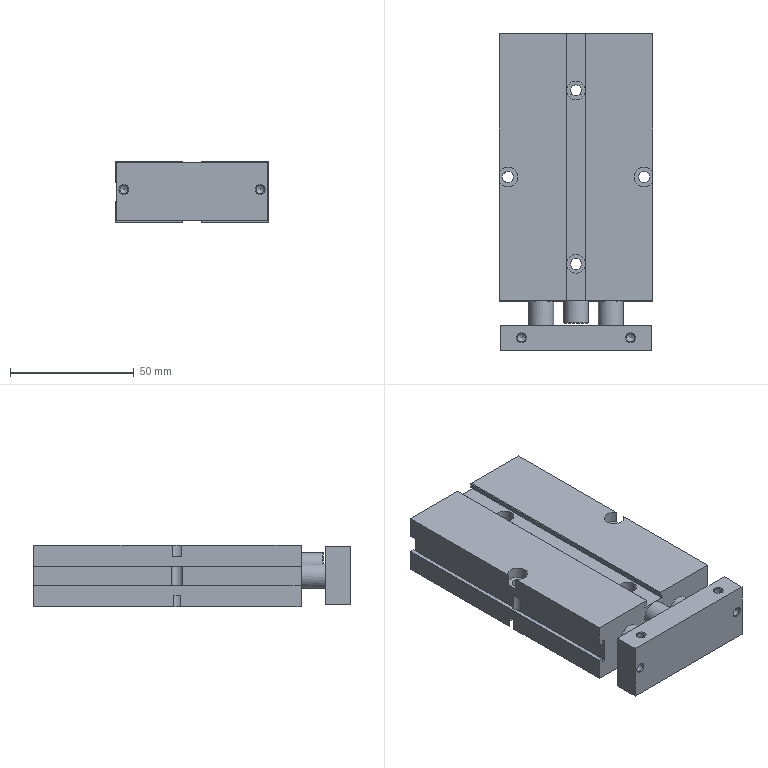Part | NX | features EXTRUDE 10, DATUM_CSYS 9, SKETCH 9, SIMPLE HOLE 8, SYMBOLIC_THREAD 8, HOLE PACKAGE 4, BLEND 1 | 5 solids | 129 faces | box 62 x 128 x 25 mm | volume 171268 mm3 | plane 57 | cylinder 55 | cone 16 | torus 1 | commonest cylinder face diameters 0.4 x30 3.3 x8 7.5 x6 4.5 x4 10 x3 8 x2